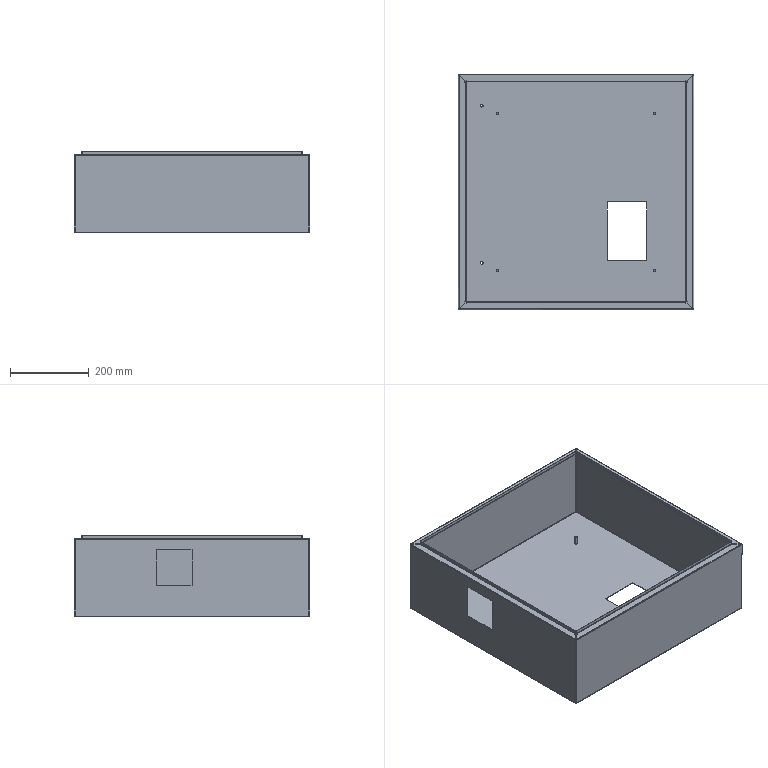Part | SolidWorks | features ICE 4, EdgeFlange 3, FlatPattern 1, HoleWzd 1, SMBaseFlange 1, SheetMetal 1 | 1 solid | 150 faces | box 600 x 600 x 208.5 mm | volume 1302353 mm3 | plane 98 | cylinder 36 | spline 16 | commonest cylinder face diameters 1.473 x12 4.473 x12 6 x8 7 x4